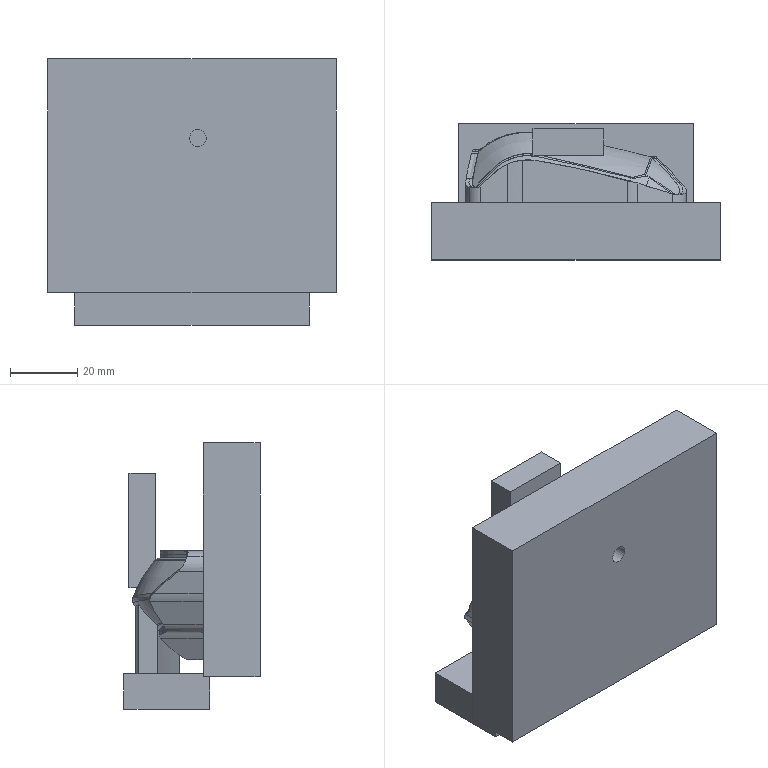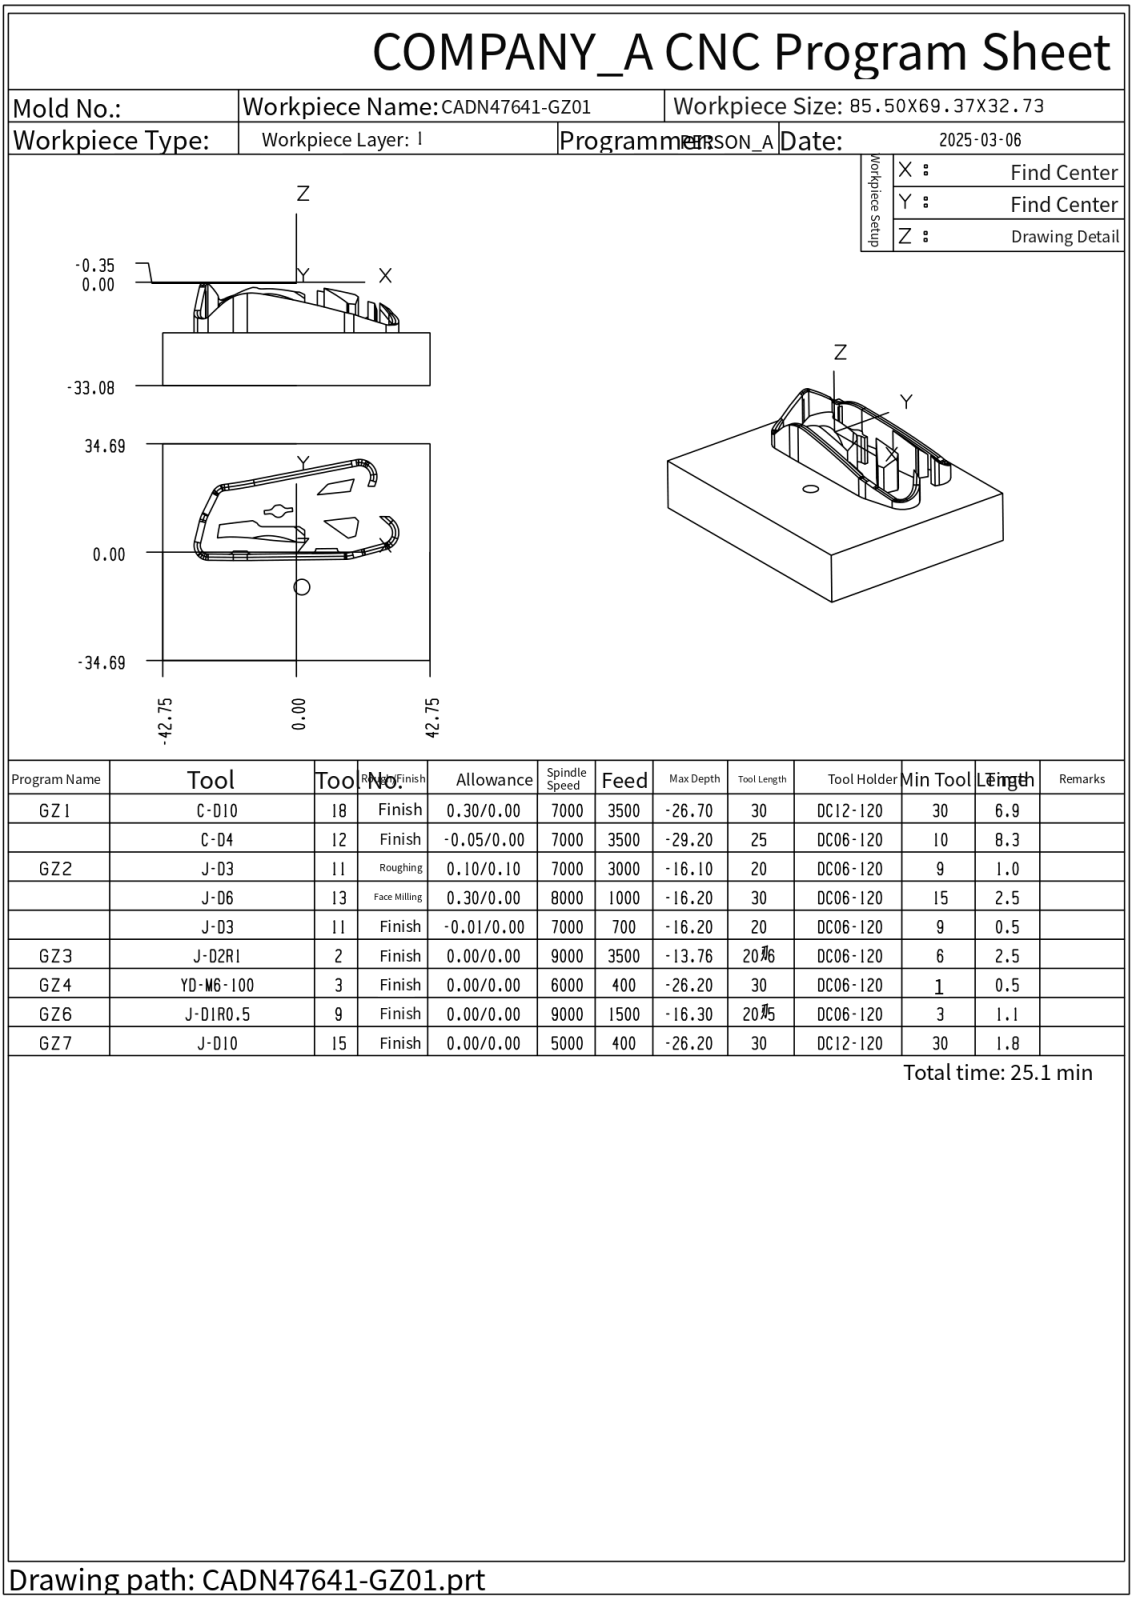NC program | NX | posted by the shop | part box 85.5 x 40.385 x 79 mm
Lines 44509 to 45221 of 71032:
44508 TOOL CALL 21 Z S9000
44509 CALL LBL101
44510 M3 M8
44511 M51
44512 CYCL DEF 32.0 TOLERANCE
44513 CYCL DEF 32.1 T0.012
44514 CYCL DEF 32.2 HSC-MODE:0
44515 L M126
44516 PLANE SPATIAL SPA-90. SPB+0.0 SPC+180. TURN FMAX SEQ-
44517 L X-30.9679 Y2.0502 FMAX
44518 L Z102.5 FMAX
44519 L Z13.2283 FMAX
44520 L Z9.372 F3500.
44521 CC X-31.7628 Y3.3223
44522 C X-30.4907 Y4.1172 DR+
44523 L X-30.5277 Y4.1763 Z9.385
44524 L X-30.665 Y4.3961 Z9.4161
44525 L X-30.8023 Y4.6158 Z9.4216
44526 L X-30.9396 Y4.8355 Z9.4012
44527 L X-31.0769 Y5.0552 Z9.3598
44528 L X-31.2141 Y5.2749 Z9.2972
44529 L X-31.3514 Y5.4946 Z9.2127
44530 L X-31.626 Y5.9341 Z8.9806
44531 L X-31.6675 Y6.0005 Z8.9386
44532 L X-31.6765 Y6.0293 Z8.9297
44533 L X-31.7057 Y6.1455 Z8.9003
44534 L X-31.7518 Y6.3749 Z8.8423
44535 L X-31.776 Y6.5505 Z8.7975
44536 L X-31.7501 Y6.509 Z8.8315
44537 L X-31.5416 Y6.1754 Z9.0732
44538 L X-31.3332 Y5.8418 Z9.2706
44539 L X-31.1247 Y5.5082 Z9.4264
44540 L X-30.9162 Y5.1746 Z9.5345
44541 L X-30.7078 Y4.841 Z9.5966
44542 L X-30.4993 Y4.5073 Z9.6037
44543 L X-30.2908 Y4.1737 Z9.5569
44544 L X-30.0824 Y3.8401 Z9.4512
44545 L X-30.054 Y3.7948 Z9.433
44546 L X-29.9789 Y3.7401 Z9.4348
44547 L X-29.7036 Y3.6104 Z9.4728
44548 L X-29.8525 Y3.8487 Z9.5866
44549 L X-29.9819 Y4.0558 Z9.6622
44550 L X-30.1113 Y4.2629 Z9.7178
44551 L X-30.2407 Y4.4699 Z9.7523
44552 L X-30.3701 Y4.677 Z9.7663
44553 L X-30.4994 Y4.884 Z9.7525
44554 L X-30.7582 Y5.2981 Z9.677
44555 L X-31.017 Y5.7122 Z9.5343
44556 L X-31.2757 Y6.1263 Z9.3258
44557 L X-31.5345 Y6.5404 Z9.0508
44558 L X-31.7932 Y6.9545 Z8.7055
44559 L X-31.8154 Y6.99 Z8.6715
44560 L X-31.8199 Y7.0661 Z8.6447
44561 L X-31.8155 Y7.3666 Z8.5506
44562 L X-31.796 Y7.3353 Z8.583
44563 L X-31.6467 Y7.0964 Z8.8151
44564 L X-31.4974 Y6.8576 Z9.01
44565 L X-31.3482 Y6.6187 Z9.1978
44566 L X-31.1989 Y6.3798 Z9.3555
44567 L X-30.9003 Y5.902 Z9.6208
44568 L X-30.7511 Y5.6631 Z9.7189
44569 L X-30.6018 Y5.4243 Z9.7951
44570 L X-30.3033 Y4.9465 Z9.885
44571 L X-30.154 Y4.7076 Z9.891
44572 L X-30.0047 Y4.4687 Z9.8729
44573 L X-29.8555 Y4.2298 Z9.8217
44574 L X-29.7062 Y3.991 Z9.7463
44575 L X-29.5569 Y3.7521 Z9.642
44576 L X-29.39 Y3.485 Z9.4963
44577 L X-29.2882 Y3.4458
44578 L X-29.082 Y3.3685 Z9.4901
44579 L X-29.1009 Y3.3988 Z9.5079
44580 L X-29.2677 Y3.6657 Z9.6717
44581 L X-29.4346 Y3.9327 Z9.8005
44582 L X-29.6014 Y4.1997 Z9.8984
44583 L X-29.7682 Y4.4666 Z9.9641
44584 L X-29.935 Y4.7336 Z9.9957
44585 L X-30.1018 Y5.0005 Z9.9978
44586 L X-30.2686 Y5.2675 Z9.9607
44587 L X-30.4354 Y5.5344 Z9.8971
44588 L X-30.6024 Y5.8017 Z9.8061
44589 L X-30.7694 Y6.0689 Z9.6876
44590 L X-30.9364 Y6.3362 Z9.5492
44591 L X-31.1034 Y6.6034 Z9.3862
44592 L X-31.4374 Y7.1379 Z8.9807
44593 L X-31.6044 Y7.4052 Z8.7378
44594 L X-31.7714 Y7.6725 Z8.4673
44595 L X-31.789 Y7.7006 Z8.4368
44596 L X-31.7839 Y7.7574 Z8.4155
44597 L X-31.7428 Y8.0032 Z8.3261
44598 L X-31.5436 Y7.6843 Z8.6698
44599 L X-31.3604 Y7.3911 Z8.9411
44600 L X-31.1772 Y7.0979 Z9.18
44601 L X-30.9939 Y6.8047 Z9.4004
44602 L X-30.8107 Y6.5115 Z9.5893
44603 L X-30.6275 Y6.2183 Z9.7481
44604 L X-30.4443 Y5.925 Z9.8763
44605 L X-30.2611 Y5.6318 Z9.9758
44606 L X-30.0778 Y5.3386 Z10.0451
44607 L X-29.8946 Y5.0454 Z10.0828
44608 L X-29.7114 Y4.7522 Z10.0805
44609 L X-29.5282 Y4.459 Z10.0326
44610 L X-29.345 Y4.1658 Z9.9516
44611 L X-29.1617 Y3.8725 Z9.8318
44612 L X-28.9785 Y3.5793 Z9.6781
44613 L X-28.7769 Y3.2567 Z9.4548
44614 L X-28.5975 Y3.1751 Z9.409
44615 L X-28.4262 Y3.0718 Z9.3318
44616 L X-28.6507 Y3.4312 Z9.6183
44617 L X-28.8519 Y3.7531 Z9.8122
44618 L X-29.053 Y4.075 Z9.959
44619 L X-29.2542 Y4.3969 Z10.0669
44620 L X-29.4553 Y4.7188 Z10.1311
44621 L X-29.6564 Y5.0407 Z10.1489
44622 L X-29.8576 Y5.3626 Z10.1247
44623 L X-30.0587 Y5.6845 Z10.053
44624 L X-30.2599 Y6.0064 Z9.9472
44625 L X-30.461 Y6.3283 Z9.8016
44626 L X-30.6622 Y6.6502 Z9.6288
44627 L X-30.8633 Y6.9721 Z9.419
44628 L X-31.0645 Y7.294 Z9.178
44629 L X-31.2656 Y7.6159 Z8.9039
44630 L X-31.4668 Y7.9378 Z8.5931
44631 L X-31.6679 Y8.2597 Z8.2427
44632 L X-31.6823 Y8.2827 Z8.215
44633 L X-31.6361 Y8.4486 Z8.1444
44634 L X-31.6058 Y8.5367 Z8.1109
44635 L X-31.3753 Y8.1679 Z8.5278
44636 L X-31.1585 Y7.8209 Z8.8652
44637 L X-30.9417 Y7.4739 Z9.1631
44638 L X-30.7249 Y7.127 Z9.428
44639 L X-30.5081 Y6.78 Z9.6543
44640 L X-30.2913 Y6.433 Z9.8449
44641 L X-30.0744 Y6.086 Z9.9951
44642 L X-29.8576 Y5.7391 Z10.1054
44643 L X-29.6408 Y5.3921 Z10.1828
44644 L X-29.424 Y5.0451 Z10.1995
44645 L X-29.2072 Y4.6982 Z10.1606
44646 L X-28.9904 Y4.3512 Z10.082
44647 L X-28.7736 Y4.0042 Z9.9539
44648 L X-28.5568 Y3.6572 Z9.7841
44649 L X-28.34 Y3.3103 Z9.5512
44650 L X-28.2315 Y3.1368 Z9.4069
44651 L X-28.1155 Y2.9511 Z9.2224
44652 L X-28.1079 Y2.939 Z9.2097
44653 L X-28.0262 Y2.9188 Z9.184
44654 L X-27.9068 Y2.8787 Z9.1335
44655 L X-27.8202 Y2.8549 Z9.1021
44656 L X-27.9506 Y3.0636 Z9.3341
44657 L X-28.0654 Y3.2473 Z9.5093
44658 L X-28.1801 Y3.431 Z9.6533
44659 L X-28.2949 Y3.6146 Z9.769
44660 L X-28.5245 Y3.982 Z9.9659
44661 L X-28.754 Y4.3494 Z10.0914
44662 L X-28.9836 Y4.7167 Z10.184
44663 L X-29.2131 Y5.0841 Z10.2248
44664 L X-29.4427 Y5.4514 Z10.214
44665 L X-29.6722 Y5.8188 Z10.1397
44666 L X-29.9018 Y6.1861 Z10.019
44667 L X-30.1313 Y6.5535 Z9.8555
44668 L X-30.3609 Y6.9208 Z9.6534
44669 L X-30.5904 Y7.2882 Z9.4059
44670 L X-30.82 Y7.6555 Z9.1249
44671 L X-31.0495 Y8.0229 Z8.8048
44672 L X-31.1643 Y8.2066 Z8.6374
44673 L X-31.2791 Y8.3903 Z8.4413
44674 L X-31.3938 Y8.5739 Z8.2493
44675 L X-31.5222 Y8.7794 Z7.9998
44676 L X-31.5172 Y8.7942 Z7.9925
44677 L X-31.4265 Y9.0026 Z7.8951
44678 L X-31.4136 Y8.9821 Z7.9215
44679 L X-31.1723 Y8.5958 Z8.3678
44680 L X-30.9309 Y8.2096 Z8.7488
44681 L X-30.6896 Y7.8233 Z9.0847
44682 L X-30.4482 Y7.4371 Z9.3835
44683 L X-30.2069 Y7.0508 Z9.6374
44684 L X-29.9655 Y6.6646 Z9.856
44685 L X-29.7241 Y6.2783 Z10.0282
44686 L X-29.4828 Y5.8921 Z10.1539
44687 L X-29.3621 Y5.6989 Z10.2019
44688 L X-29.2414 Y5.5058 Z10.2274
44689 L X-29.0001 Y5.1196 Z10.2376
44690 L X-28.7587 Y4.7333 Z10.1876
44691 L X-28.5174 Y4.3471 Z10.0948
44692 L X-28.276 Y3.9608 Z9.9543
44693 L X-28.1553 Y3.7677 Z9.8637
44694 L X-28.0346 Y3.5746 Z9.7499
44695 L X-27.914 Y3.3814 Z9.6122
44696 L X-27.7933 Y3.1883 Z9.4387
44697 L X-27.544 Y2.7894 Z9.0183
44698 L X-27.5361 Y2.7767 Z9.0037
44699 L X-27.2498 Y2.695 Z8.9022
44700 L X-27.2657 Y2.7204 Z8.9316
44701 L X-27.5187 Y3.1252 Z9.3473
44702 L X-27.6451 Y3.3276 Z9.539
44703 L X-27.7716 Y3.5301 Z9.7026
44704 L X-27.8981 Y3.7325 Z9.8305
44705 L X-28.0246 Y3.9349 Z9.9346
44706 L X-28.2776 Y4.3398 Z10.0886
44707 L X-28.5306 Y4.7447 Z10.1759
44708 L X-28.7836 Y5.1495 Z10.2294
44709 L X-29.0366 Y5.5544 Z10.2264
44710 L X-29.1631 Y5.7568 Z10.2005
44711 L X-29.2896 Y5.9592 Z10.1506
44712 L X-29.5425 Y6.3641 Z10.0162
44713 L X-29.7955 Y6.769 Z9.8374
44714 L X-30.0485 Y7.1738 Z9.6167
44715 L X-30.3015 Y7.5787 Z9.3445
44716 L X-30.5545 Y7.9836 Z9.032
44717 L X-30.8075 Y8.3884 Z8.6787
44718 L X-31.0604 Y8.7933 Z8.2772
44719 L X-31.1869 Y8.9957 Z8.0562
44720 L X-31.3256 Y9.2175 Z7.7822
44721 L X-31.215 Y9.4171 Z7.6741
44722 L X-31.2029 Y9.3977 Z7.6994
44723 L X-30.9391 Y8.9756 Z8.1917
44724 L X-30.6754 Y8.5535 Z8.6017
44725 L X-30.4116 Y8.1314 Z8.9687
44726 L X-30.1478 Y7.7092 Z9.2987
44727 L X-29.8841 Y7.2871 Z9.5762
44728 L X-29.6203 Y6.865 Z9.8092
44729 L X-29.3565 Y6.4429 Z9.9955
44730 L X-29.0928 Y6.0208 Z10.1351
44731 L X-28.9609 Y5.8097 Z10.1798
44732 L X-28.829 Y5.5986 Z10.2036
44733 L X-28.5652 Y5.1765 Z10.2076
44734 L X-28.3015 Y4.7544 Z10.1592
44735 L X-28.0377 Y4.3323 Z10.0643
44736 L X-27.9058 Y4.1212 Z9.9964
44737 L X-27.7739 Y3.9102 Z9.9023
44738 L X-27.642 Y3.6991 Z9.7792
44739 L X-27.5102 Y3.4881 Z9.6312
44740 L X-27.2464 Y3.0659 Z9.2667
44741 L X-26.9826 Y2.6438 Z8.8361
44742 L X-26.9671 Y2.619 Z8.8073
44743 L X-26.8707 Y2.5933 Z8.7752
44744 L X-26.6874 Y2.5478 Z8.718
44745 L X-26.7026 Y2.5722 Z8.7464
44746 L X-26.9767 Y3.0108 Z9.1901
44747 L X-27.2508 Y3.4495 Z9.5494
44748 L X-27.3879 Y3.6688 Z9.7129
44749 L X-27.525 Y3.8882 Z9.8496
44750 L X-27.7991 Y4.3268 Z10.0368
44751 L X-28.0732 Y4.7655 Z10.1345
44752 L X-28.3473 Y5.2041 Z10.1718
44753 L X-28.6214 Y5.6428 Z10.1724
44754 L X-28.7584 Y5.8621 Z10.1468
44755 L X-28.8955 Y6.0815 Z10.0984
44756 L X-29.1696 Y6.5201 Z9.9495
44757 L X-29.4437 Y6.9588 Z9.7616
44758 L X-29.7178 Y7.3975 Z9.525
44759 L X-29.9919 Y7.8361 Z9.2359
44760 L X-30.266 Y8.2748 Z8.8964
44761 L X-30.5401 Y8.7134 Z8.5183
44762 L X-30.8142 Y9.1521 Z8.0938
44763 L X-31.0883 Y9.5908 Z7.5863
44764 L X-31.1001 Y9.6097 Z7.5614
44765 L X-31.015 Y9.7354 Z7.4842
44766 L X-30.9759 Y9.7873 Z7.4522
44767 L X-30.9646 Y9.7691 Z7.4761
44768 L X-30.6809 Y9.3152 Z7.9958
44769 L X-30.3972 Y8.8612 Z8.4268
44770 L X-30.1135 Y8.4072 Z8.8154
44771 L X-29.8298 Y7.9532 Z9.1565
44772 L X-29.5462 Y7.4992 Z9.4564
44773 L X-29.2625 Y7.0452 Z9.6942
44774 L X-28.9788 Y6.5913 Z9.8912
44775 L X-28.6951 Y6.1373 Z10.0436
44776 L X-28.5533 Y5.9103 Z10.0921
44777 L X-28.4115 Y5.6833 Z10.12
44778 L X-28.1278 Y5.2293 Z10.1303
44779 L X-27.8441 Y4.7753 Z10.093
44780 L X-27.7023 Y4.5484 Z10.0549
44781 L X-27.5604 Y4.3214 Z9.9895
44782 L X-27.2767 Y3.8674 Z9.7831
44783 L X-26.9931 Y3.4134 Z9.4793
44784 L X-26.7094 Y2.9594 Z9.1162
44785 L X-26.4257 Y2.5054 Z8.6623
44786 L X-26.4107 Y2.4814 Z8.6343
44787 L X-26.18 Y2.4285 Z8.5675
44788 L X-26.1379 Y2.4213 Z8.5582
44789 L X-26.1521 Y2.444 Z8.5842
44790 L X-26.2983 Y2.6781 Z8.8272
44791 L X-26.4446 Y2.9121 Z9.045
44792 L X-26.5909 Y3.1462 Z9.2421
44793 L X-26.7371 Y3.3802 Z9.4149
44794 L X-26.8834 Y3.6143 Z9.5664
44795 L X-27.0296 Y3.8484 Z9.7066
44796 L X-27.1759 Y4.0824 Z9.8295
44797 L X-27.3221 Y4.3165 Z9.9281
44798 L X-27.6147 Y4.7846 Z10.0475
44799 L X-27.9072 Y5.2527 Z10.0777
44800 L X-28.1997 Y5.7208 Z10.0544
44801 L X-28.3459 Y5.9549 Z10.0233
44802 L X-28.4922 Y6.189 Z9.9709
44803 L X-28.7847 Y6.6571 Z9.8109
44804 L X-29.0772 Y7.1252 Z9.6135
44805 L X-29.3697 Y7.5933 Z9.368
44806 L X-29.6623 Y8.0614 Z9.0759
44807 L X-29.9548 Y8.5296 Z8.7223
44808 L X-30.2473 Y8.9977 Z8.3344
44809 L X-30.5398 Y9.4658 Z7.8966
44810 L X-30.8323 Y9.9339 Z7.3695
44811 L X-30.8435 Y9.9518 Z7.3468
44812 L X-30.7097 Y10.1141 Z7.2304
44813 L X-30.5482 Y9.8557 Z7.5312
44814 L X-30.3979 Y9.6151 Z7.7828
44815 L X-30.0973 Y9.1341 Z8.2236
44816 L X-29.7967 Y8.653 Z8.6175
44817 L X-29.4961 Y8.1719 Z8.9685
44818 L X-29.1955 Y7.6908 Z9.264
44819 L X-28.8948 Y7.2097 Z9.502
44820 L X-28.5942 Y6.7287 Z9.7073
44821 L X-28.2936 Y6.2476 Z9.8759
44822 L X-28.1433 Y6.007 Z9.9366
44823 L X-27.993 Y5.7665 Z9.9718
44824 L X-27.6924 Y5.2854 Z10.0138
44825 L X-27.5421 Y5.0449 Z10.011
44826 L X-27.3918 Y4.8043 Z9.9859
44827 L X-27.0912 Y4.3233 Z9.8624
44828 L X-26.9409 Y4.0827 Z9.7583
44829 L X-26.8657 Y3.9624 Z9.7005
44830 L X-26.6402 Y3.6016 Z9.5096
44831 L X-26.4899 Y3.3611 Z9.3586
44832 L X-26.1893 Y2.88 Z8.9877
44833 L X-26.039 Y2.6395 Z8.7698
44834 L X-25.8745 Y2.3762 Z8.4958
44835 L X-25.8346 Y2.3694 Z8.4864
44836 L X-25.5922 Y2.3009 Z8.4056
44837 L X-25.7626 Y2.5736 Z8.6894
44838 L X-25.9172 Y2.821 Z8.9085
44839 L X-26.2265 Y3.316 Z9.2835
44840 L X-26.3811 Y3.5634 Z9.4364
44841 L X-26.5358 Y3.8109 Z9.5637
44842 L X-26.845 Y4.3058 Z9.7789
44843 L X-26.9997 Y4.5533 Z9.8549
44844 L X-27.1543 Y4.8008 Z9.9088
44845 L X-27.4636 Y5.2957 Z9.9402
44846 L X-27.7728 Y5.7906 Z9.8871
44847 L X-28.0821 Y6.2855 Z9.7733
44848 L X-28.3914 Y6.7805 Z9.5897
44849 L X-28.7006 Y7.2754 Z9.3818
44850 L X-29.0099 Y7.7703 Z9.1453
44851 L X-29.3192 Y8.2653 Z8.8579
44852 L X-29.6284 Y8.7602 Z8.5046
44853 L X-29.9377 Y9.2551 Z8.1094
44854 L X-30.247 Y9.7501 Z7.6749
44855 L X-30.4016 Y9.9975 Z7.4235
44856 L X-30.5671 Y10.2623 Z7.1195
44857 L X-30.4198 Y10.4031 Z7.0073
44858 L X-30.409 Y10.3857 Z7.0285
44859 L X-30.25 Y10.1313 Z7.3118
44860 L X-30.091 Y9.8769 Z7.5585
44861 L X-29.7731 Y9.3681 Z7.9912
44862 L X-29.4551 Y8.8592 Z8.3848
44863 L X-29.1371 Y8.3504 Z8.7342
44864 L X-28.8192 Y7.8415 Z9.0059
44865 L X-28.5012 Y7.3327 Z9.2387
44866 L X-28.1833 Y6.8239 Z9.4517
44867 L X-27.8653 Y6.315 Z9.6594
44868 L X-27.5473 Y5.8062 Z9.7909
44869 L X-27.3884 Y5.5517 Z9.8328
44870 L X-27.2294 Y5.2973 Z9.8543
44871 L X-26.9114 Y4.7885 Z9.8246
44872 L X-26.7524 Y4.5341 Z9.7673
44873 L X-26.673 Y4.4068 Z9.7309
44874 L X-26.5935 Y4.2796 Z9.6904
44875 L X-26.4345 Y4.0252 Z9.6003
44876 L X-26.2755 Y3.7708 Z9.4863
44877 L X-26.1165 Y3.5164 Z9.3575
44878 L X-25.9575 Y3.262 Z9.2021
44879 L X-25.6396 Y2.7531 Z8.826
44880 L X-25.4806 Y2.4987 Z8.6017
44881 L X-25.3058 Y2.2189 Z8.3103
44882 L X-25.2015 Y2.1888 Z8.2755
44883 L X-25.0224 Y2.1418 Z8.2205
44884 L X-25.201 Y2.4277 Z8.5177
44885 L X-25.3641 Y2.6888 Z8.7472
44886 L X-25.5273 Y2.9499 Z8.9474
44887 L X-25.6905 Y3.211 Z9.1226
44888 L X-25.8536 Y3.4721 Z9.2798
44889 L X-26.0168 Y3.7332 Z9.4109
44890 L X-26.1799 Y3.9943 Z9.5223
44891 L X-26.3431 Y4.2554 Z9.6111
44892 L X-26.6694 Y4.7776 Z9.7337
44893 L X-26.8325 Y5.0387 Z9.7573
44894 L X-26.9957 Y5.2998 Z9.7583
44895 L X-27.1589 Y5.5609 Z9.7316
44896 L X-27.322 Y5.822 Z9.6824
44897 L X-27.4852 Y6.0831 Z9.6147
44898 L X-27.6483 Y6.3442 Z9.5262
44899 L X-27.9746 Y6.8664 Z9.2992
44900 L X-28.301 Y7.3886 Z9.0821
44901 L X-28.6273 Y7.9108 Z8.8593
44902 L X-28.9536 Y8.433 Z8.5915
44903 L X-29.1167 Y8.6942 Z8.4354
44904 L X-29.2799 Y8.9553 Z8.2522
44905 L X-29.6062 Y9.4775 Z7.8605
44906 L X-29.9325 Y9.9997 Z7.4383
44907 L X-30.0957 Y10.2608 Z7.1916
44908 L X-30.2695 Y10.5389 Z6.8891
44909 L X-30.1093 Y10.659 Z6.7776
44910 L X-29.9317 Y10.3748 Z7.0758
44911 L X-29.7648 Y10.1077 Z7.3144
44912 L X-29.4309 Y9.5733 Z7.7237
44913 L X-29.097 Y9.039 Z8.1172
44914 L X-28.9301 Y8.7718 Z8.292
44915 L X-28.7631 Y8.5047 Z8.4446
44916 L X-28.4292 Y7.9703 Z8.6962
44917 L X-28.0953 Y7.436 Z8.9105
44918 L X-27.7614 Y6.9017 Z9.1344
44919 L X-27.4276 Y6.3673 Z9.3862
44920 L X-27.0937 Y5.833 Z9.5646
44921 L X-26.9267 Y5.5658 Z9.6236
44922 L X-26.7598 Y5.2987 Z9.6592
44923 L X-26.5928 Y5.0315 Z9.6609
44924 L X-26.5094 Y4.8979 Z9.6523
44925 L X-26.2589 Y4.4972 Z9.596
44926 L X-26.092 Y4.23 Z9.5306
44927 L X-25.9251 Y3.9628 Z9.4435
44928 L X-25.7581 Y3.6957 Z9.3347
44929 L X-25.4242 Y3.1613 Z9.0496
44930 L X-25.2573 Y2.8942 Z8.8735
44931 L X-25.0903 Y2.627 Z8.6704
44932 L X-24.9234 Y2.3598 Z8.4367
44933 L X-24.741 Y2.0679 Z8.1342
44934 L X-24.459 Y1.9931 Z8.048
44935 L X-24.6452 Y2.2911 Z8.3547
44936 L X-24.8159 Y2.5643 Z8.5926
44937 L X-24.9866 Y2.8375 Z8.7988
44938 L X-25.1573 Y3.1107 Z8.976
44939 L X-25.328 Y3.3839 Z9.1293
44940 L X-25.4988 Y3.6571 Z9.2574
44941 L X-25.6695 Y3.9303 Z9.3647
44942 L X-25.8402 Y4.2035 Z9.4495
44943 L X-26.0109 Y4.4767 Z9.5122
44944 L X-26.1816 Y4.7499 Z9.5463
44945 L X-26.3523 Y5.023 Z9.5627
44946 L X-26.523 Y5.2962 Z9.5557
44947 L X-26.6938 Y5.5694 Z9.5127
44948 L X-26.8645 Y5.8426 Z9.4391
44949 L X-27.2059 Y6.389 Z9.2315
44950 L X-27.5473 Y6.9354 Z8.9632
44951 L X-27.8888 Y7.4818 Z8.7278
44952 L X-28.2302 Y8.0282 Z8.5218
44953 L X-28.5716 Y8.5746 Z8.2878
44954 L X-28.7423 Y8.8478 Z8.1407
44955 L X-28.913 Y9.121 Z7.9723
44956 L X-29.2545 Y9.6674 Z7.5752
44957 L X-29.5959 Y10.2138 Z7.1817
44958 L X-29.7666 Y10.487 Z6.9488
44959 L X-29.9479 Y10.7772 Z6.6566
44960 L X-29.8099 Y10.8679 Z6.5579
44961 L X-29.7801 Y10.8851 Z6.5379
44962 L X-29.7695 Y10.8681 Z6.5557
44963 L X-29.5952 Y10.5891 Z6.8204
44964 L X-29.4208 Y10.3101 Z7.042
44965 L X-29.0721 Y9.752 Z7.424
44966 L X-28.8978 Y9.473 Z7.6285
44967 L X-28.7234 Y9.194 Z7.8201
44968 L X-28.549 Y8.915 Z7.988
44969 L X-28.3747 Y8.6359 Z8.1233
44970 L X-28.026 Y8.0779 Z8.3381
44971 L X-27.6773 Y7.5199 Z8.5332
44972 L X-27.3286 Y6.9618 Z8.7795
44973 L X-26.9799 Y6.4038 Z9.067
44974 L X-26.6312 Y5.8457 Z9.3159
44975 L X-26.4568 Y5.5667 Z9.4011
44976 L X-26.2825 Y5.2877 Z9.4479
44977 L X-26.1081 Y5.0087 Z9.4668
44978 L X-25.9338 Y4.7297 Z9.4568
44979 L X-25.7594 Y4.4506 Z9.4262
44980 L X-25.5851 Y4.1716 Z9.3659
44981 L X-25.2364 Y3.6136 Z9.1818
44982 L X-25.062 Y3.3346 Z9.0532
44983 L X-24.8877 Y3.0555 Z8.8998
44984 L X-24.7133 Y2.7765 Z8.7208
44985 L X-24.539 Y2.4975 Z8.5114
44986 L X-24.3646 Y2.2185 Z8.2691
44987 L X-24.1746 Y1.9144 Z7.9591
44988 L X-24.0575 Y1.882 Z7.9228
44989 L X-23.8875 Y1.8314 Z7.8671
44990 L X-24.0814 Y2.1417 Z8.1843
44991 L X-24.2593 Y2.4263 Z8.4265
44992 L X-24.4372 Y2.711 Z8.6394
44993 L X-24.6151 Y2.9957 Z8.8207
44994 L X-24.7929 Y3.2804 Z8.9746
44995 L X-24.9708 Y3.565 Z9.1037
44996 L X-25.1487 Y3.8497 Z9.2055
44997 L X-25.3266 Y4.1344 Z9.2811
44998 L X-25.5045 Y4.419 Z9.3384
44999 L X-25.6823 Y4.7037 Z9.3638
45000 L X-25.8602 Y4.9884 Z9.3719
45001 L X-26.0381 Y5.2731 Z9.3434
45002 L X-26.216 Y5.5577 Z9.2866
45003 L X-26.3939 Y5.8424 Z9.194
45004 L X-26.5718 Y6.1271 Z9.0622
45005 L X-26.7496 Y6.4117 Z8.9037
45006 L X-26.9275 Y6.6964 Z8.7374
45007 L X-27.1054 Y6.9811 Z8.5856
45008 L X-27.2833 Y7.2658 Z8.445
45009 L X-27.4612 Y7.5504 Z8.3328
45010 L X-27.8169 Y8.1198 Z8.1527
45011 L X-28.1727 Y8.6891 Z7.9552
45012 L X-28.3506 Y8.9738 Z7.8295
45013 L X-28.5285 Y9.2584 Z7.6729
45014 L X-28.8842 Y9.8278 Z7.2692
45015 L X-29.24 Y10.3971 Z6.8979
45016 L X-29.4179 Y10.6818 Z6.6886
45017 L X-29.5958 Y10.9665 Z6.4364
45018 L X-29.6064 Y10.9835 Z6.4194
45019 L X-29.4278 Y11.0741 Z6.2977
45020 L X-29.4171 Y11.057 Z6.3135
45021 L X-29.2358 Y10.7669 Z6.5523
45022 L X-29.0545 Y10.4767 Z6.7485
45023 L X-28.8731 Y10.1865 Z6.9207
45024 L X-28.6918 Y9.8963 Z7.1159
45025 L X-28.5105 Y9.6061 Z7.3316
45026 L X-28.3292 Y9.3159 Z7.5169
45027 L X-28.1478 Y9.0257 Z7.6662
45028 L X-27.9665 Y8.7355 Z7.7827
45029 L X-27.6038 Y8.1552 Z7.963
45030 L X-27.2412 Y7.5748 Z8.1369
45031 L X-27.0598 Y7.2846 Z8.2473
45032 L X-26.8785 Y6.9944 Z8.3878
45033 L X-26.8332 Y6.9219 Z8.4289
45034 L X-26.6745 Y6.668 Z8.586
45035 L X-26.5159 Y6.414 Z8.7468
45036 L X-26.3345 Y6.1239 Z8.9271
45037 L X-26.1532 Y5.8337 Z9.0719
45038 L X-25.9719 Y5.5435 Z9.176
45039 L X-25.7905 Y5.2533 Z9.2404
45040 L X-25.6092 Y4.9631 Z9.2757
45041 L X-25.4279 Y4.6729 Z9.2715
45042 L X-25.2466 Y4.3827 Z9.2495
45043 L X-25.0652 Y4.0926 Z9.1996
45044 L X-24.8839 Y3.8024 Z9.1253
45045 L X-24.7026 Y3.5122 Z9.0235
45046 L X-24.5212 Y3.222 Z8.894
45047 L X-24.3399 Y2.9318 Z8.7391
45048 L X-24.1586 Y2.6416 Z8.5551
45049 L X-23.9773 Y2.3514 Z8.3437
45050 L X-23.7959 Y2.0612 Z8.097
45051 L X-23.5986 Y1.7454 Z7.7733
45052 L X-23.4171 Y1.6914 Z7.7146
45053 L X-23.3123 Y1.6637 Z7.6842
45054 L X-23.5126 Y1.9842 Z8.013
45055 L X-23.6974 Y2.28 Z8.2643
45056 L X-23.8822 Y2.5758 Z8.4787
45057 L X-24.067 Y2.8715 Z8.6597
45058 L X-24.2518 Y3.1673 Z8.8152
45059 L X-24.4366 Y3.463 Z8.9445
45060 L X-24.6214 Y3.7588 Z9.0459
45061 L X-24.8062 Y4.0545 Z9.1188
45062 L X-24.9911 Y4.3503 Z9.1642
45063 L X-25.1759 Y4.646 Z9.1806
45064 L X-25.3607 Y4.9418 Z9.178
45065 L X-25.5455 Y5.2375 Z9.1338
45066 L X-25.7303 Y5.5333 Z9.0621
45067 L X-25.9151 Y5.8291 Z8.9477
45068 L X-26.0999 Y6.1248 Z8.7887
45069 L X-26.5231 Y6.8021 Z8.3299
45070 L X-26.6423 Y6.9929 Z8.2062
45071 L X-26.7615 Y7.1836 Z8.0997
45072 L X-26.8554 Y7.3339 Z8.0283
45073 L X-26.9493 Y7.4842 Z7.9742
45074 L X-27.1371 Y7.7847 Z7.8816
45075 L X-27.4502 Y8.2857 Z7.7473
45076 L X-27.7632 Y8.7866 Z7.6045
45077 L X-27.948 Y9.0824 Z7.496
45078 L X-28.1328 Y9.3781 Z7.3559
45079 L X-28.3176 Y9.6739 Z7.1774
45080 L X-28.5024 Y9.9696 Z6.9587
45081 L X-28.5948 Y10.1175 Z6.8426
45082 L X-28.6872 Y10.2654 Z6.7525
45083 L X-28.872 Y10.5611 Z6.5887
45084 L X-29.0568 Y10.8569 Z6.4078
45085 L X-29.2416 Y11.1526 Z6.1801
45086 L X-29.2522 Y11.1696 Z6.1651
45087 L X-29.1849 Y11.2135 Z6.1044
45088 L X-29.0865 Y11.2809 Z6.0122
45089 L X-29.0759 Y11.2639 Z6.0265
45090 L X-28.8875 Y10.9623 Z6.2475
45091 L X-28.6991 Y10.6608 Z6.4139
45092 L X-28.5106 Y10.3592 Z6.5664
45093 L X-28.4164 Y10.2084 Z6.6646
45094 L X-28.3222 Y10.0577 Z6.786
45095 L X-28.1338 Y9.7561 Z7.0058
45096 L X-27.9453 Y9.4545 Z7.1782
45097 L X-27.7569 Y9.153 Z7.3091
45098 L X-27.5684 Y8.8514 Z7.4179
45099 L X-27.322 Y8.4569 Z7.5168
45100 L X-27.0755 Y8.0625 Z7.576
45101 L X-26.829 Y7.668 Z7.6556
45102 L X-26.7057 Y7.4708 Z7.7125
45103 L X-26.6749 Y7.4214 Z7.7312
45104 L X-26.6441 Y7.3721 Z7.7534
45105 L X-26.5825 Y7.2735 Z7.8061
45106 L X-25.8725 Y6.1374 Z8.6406
45107 L X-25.6841 Y5.8358 Z8.8153
45108 L X-25.4956 Y5.5342 Z8.9423
45109 L X-25.3072 Y5.2327 Z9.0279
45110 L X-25.1188 Y4.9311 Z9.0773
45111 L X-24.9303 Y4.6296 Z9.0928
45112 L X-24.7419 Y4.328 Z9.0786
45113 L X-24.5535 Y4.0264 Z9.0394
45114 L X-24.365 Y3.7249 Z8.9687
45115 L X-24.1766 Y3.4233 Z8.8685
45116 L X-23.9882 Y3.1217 Z8.7408
45117 L X-23.7997 Y2.8202 Z8.5903
45118 L X-23.6113 Y2.5186 Z8.4083
45119 L X-23.4228 Y2.2171 Z8.1915
45120 L X-23.2344 Y1.9155 Z7.9365
45121 L X-23.0305 Y1.5892 Z7.6026
45122 L X-22.7478 Y1.5133 Z7.5206
45123 L X-22.9557 Y1.846 Z7.8592
45124 L X-23.1479 Y2.1534 Z8.118
45125 L X-23.34 Y2.4609 Z8.3372
45126 L X-23.5321 Y2.7684 Z8.5207
45127 L X-23.7243 Y3.0759 Z8.6708
45128 L X-23.9164 Y3.3833 Z8.7921
45129 L X-24.1085 Y3.6908 Z8.8906
45130 L X-24.3007 Y3.9983 Z8.9589
45131 L X-24.4928 Y4.3058 Z8.9918
45132 L X-24.6849 Y4.6133 Z9.0038
45133 L X-24.8771 Y4.9207 Z8.9769
45134 L X-25.0692 Y5.2282 Z8.9197
45135 L X-25.2613 Y5.5357 Z8.8181
45136 L X-25.4535 Y5.8432 Z8.6783
45137 L X-25.6456 Y6.1507 Z8.4869
45138 L X-25.8377 Y6.4581 Z8.2459
45139 L X-26.0374 Y6.7776 Z7.9746
45140 L X-26.1372 Y6.9374 Z7.8154
45141 L X-26.2941 Y7.1884 Z7.4963
45142 L X-26.3727 Y7.3142 Z7.3555
45143 L X-26.4292 Y7.4046 Z7.2859
45144 L X-26.4655 Y7.4628 Z7.2574
45145 L X-26.5643 Y7.6208 Z7.2246
45146 L X-26.6993 Y7.837 Z7.2282
45147 L X-26.8344 Y8.0532 Z7.2658
45148 L X-27.1046 Y8.4856 Z7.2802
45149 L X-27.3748 Y8.918 Z7.2187
45150 L X-27.567 Y9.2255 Z7.1262
45151 L X-27.7591 Y9.5329 Z6.9955
45152 L X-27.9512 Y9.8404 Z6.8327
45153 L X-28.1434 Y10.1479 Z6.6223
45154 L X-28.2634 Y10.3401 Z6.4671
45155 L X-28.2875 Y10.3785 Z6.4377
45156 L X-28.3355 Y10.4554 Z6.3911
45157 L X-28.5276 Y10.7629 Z6.2459
45158 L X-28.7198 Y11.0703 Z6.0861
45159 L X-28.9119 Y11.3778 Z5.8679
45160 L X-28.9225 Y11.3948 Z5.8538
45161 L X-28.7633 Y11.5165 Z5.6836
45162 L X-28.7527 Y11.4994 Z5.6975
45163 L X-28.5561 Y11.1848 Z5.9168
45164 L X-28.3595 Y10.8702 Z6.0758
45165 L X-28.1628 Y10.5555 Z6.2232
45166 L X-28.1383 Y10.5162 Z6.2476
45167 L X-27.9662 Y10.2409 Z6.461
45168 L X-27.7696 Y9.9262 Z6.6669
45169 L X-27.573 Y9.6116 Z6.822
45170 L X-27.3764 Y9.297 Z6.9343
45171 L X-27.1798 Y8.9823 Z6.9975
45172 L X-27.0323 Y8.7463 Z6.999
45173 L X-26.8849 Y8.5104 Z6.9713
45174 L X-26.7374 Y8.2744 Z6.8899
45175 L X-26.6637 Y8.1564 Z6.826
45176 L X-26.59 Y8.0384 Z6.7348
45177 L X-26.4425 Y7.8024 Z6.5156
45178 L X-26.3688 Y7.6844 Z6.4594
45179 L X-26.3319 Y7.6254 Z6.4567
45180 L X-26.2951 Y7.5664 Z6.4744
45181 L X-26.2213 Y7.4484 Z6.5586
45182 L X-26.1476 Y7.3305 Z6.7211
45183 L X-26.0739 Y7.2125 Z6.9391
45184 L X-26.0001 Y7.0945 Z7.2091
45185 L X-25.9018 Y6.9371 Z7.552
45186 L X-25.8035 Y6.7798 Z7.7767
45187 L X-25.7052 Y6.6225 Z7.939
45188 L X-25.6069 Y6.4652 Z8.0781
45189 L X-25.4103 Y6.1505 Z8.34
45190 L X-25.2137 Y5.8359 Z8.5458
45191 L X-25.0171 Y5.5213 Z8.7012
45192 L X-24.8205 Y5.2066 Z8.8145
45193 L X-24.6239 Y4.892 Z8.8784
45194 L X-24.4273 Y4.5773 Z8.9136
45195 L X-24.2307 Y4.2627 Z8.9037
45196 L X-24.0341 Y3.9481 Z8.8739
45197 L X-23.8374 Y3.6334 Z8.8059
45198 L X-23.6408 Y3.3188 Z8.7113
45199 L X-23.4442 Y3.0041 Z8.5895
45200 L X-23.2476 Y2.6895 Z8.4359
45201 L X-23.051 Y2.3749 Z8.2476
45202 L X-22.8544 Y2.0602 Z8.0217
45203 L X-22.6578 Y1.7456 Z7.7542
45204 L X-22.4421 Y1.4005 Z7.4047
45205 L X-22.381 Y1.3739 Z7.3776
45206 L X-22.1416 Y1.296 Z7.2971
45207 L X-22.3593 Y1.6443 Z7.6524
45208 L X-22.5605 Y1.9663 Z7.9252
45209 L X-22.7616 Y2.2882 Z8.1576
45210 L X-22.9628 Y2.6102 Z8.351
45211 L X-23.164 Y2.9321 Z8.508
45212 L X-23.3651 Y3.254 Z8.6315
45213 L X-23.5663 Y3.576 Z8.7252
45214 L X-23.7675 Y3.8979 Z8.7885
45215 L X-23.9686 Y4.2198 Z8.8158
45216 L X-24.1698 Y4.5418 Z8.8224
45217 L X-24.371 Y4.8637 Z8.7797
45218 L X-24.5721 Y5.1856 Z8.7084
45219 L X-24.7733 Y5.5076 Z8.5842
45220 L X-24.9745 Y5.8295 Z8.415